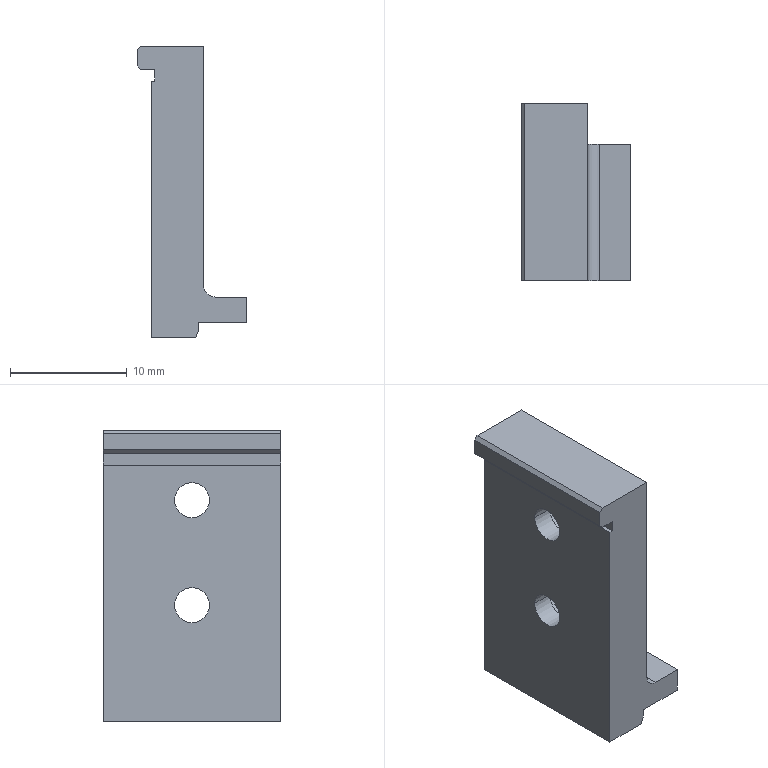Part | NX | 1 solid | 29 faces | box 9.4 x 15.2 x 25 mm | volume 1695 mm3 | plane 20 | cylinder 9 | commonest cylinder face diameters 3 x4 5 x4 2 x1
STEP:
#1=CARTESIAN_POINT('',(-1.77,0.,-1.43));
#2=VERTEX_POINT('',#1);
#3=CARTESIAN_POINT('',(-2.025,0.,-2.13));
#4=VERTEX_POINT('',#3);
#5=CARTESIAN_POINT('',(-1.25,0.,0.));
#6=DIRECTION('',(-0.342,0.,-0.9397));
#7=VECTOR('',#6,1000.);
#8=LINE('',#5,#7);
#9=EDGE_CURVE('',#2,#4,#8,.T.);
#10=ORIENTED_EDGE('',*,*,#9,.T.);
#11=CARTESIAN_POINT('',(-5.85,0.,-2.13));
#12=VERTEX_POINT('',#11);
#13=CARTESIAN_POINT('',(0.,0.,-2.13));
#14=DIRECTION('',(1.,0.,0.));
#15=VECTOR('',#14,1000.);
#16=LINE('',#13,#15);
#17=EDGE_CURVE('',#12,#4,#16,.T.);
#18=ORIENTED_EDGE('',*,*,#17,.F.);
#19=CARTESIAN_POINT('',(-5.85,0.,19.87));
#20=VERTEX_POINT('',#19);
#21=CARTESIAN_POINT('',(-5.85,0.,0.));
#22=DIRECTION('',(0.,0.,1.));
#23=VECTOR('',#22,1000.);
#24=LINE('',#21,#23);
#25=EDGE_CURVE('',#12,#20,#24,.T.);
#26=ORIENTED_EDGE('',*,*,#25,.T.);
#27=CARTESIAN_POINT('',(-5.55,0.,19.87));
#28=VERTEX_POINT('',#27);
#29=CARTESIAN_POINT('',(0.,0.,19.87));
#30=DIRECTION('',(1.,0.,0.));
#31=VECTOR('',#30,1000.);
#32=LINE('',#29,#31);
#33=EDGE_CURVE('',#20,#28,#32,.T.);
#34=ORIENTED_EDGE('',*,*,#33,.T.);
#35=CARTESIAN_POINT('',(-5.55,0.,20.87));
#36=VERTEX_POINT('',#35);
#37=CARTESIAN_POINT('',(-5.55,0.,0.));
#38=DIRECTION('',(0.,0.,1.));
#39=VECTOR('',#38,1000.);
#40=LINE('',#37,#39);
#41=EDGE_CURVE('',#28,#36,#40,.T.);
#42=ORIENTED_EDGE('',*,*,#41,.T.);
#43=CARTESIAN_POINT('',(-6.75,0.,20.87));
#44=VERTEX_POINT('',#43);
#45=CARTESIAN_POINT('',(0.,0.,20.87));
#46=DIRECTION('',(-1.,0.,0.));
#47=VECTOR('',#46,1000.);
#48=LINE('',#45,#47);
#49=EDGE_CURVE('',#36,#44,#48,.T.);
#50=ORIENTED_EDGE('',*,*,#49,.T.);
#51=CARTESIAN_POINT('',(-7.05,0.,21.17));
#52=VERTEX_POINT('',#51);
#53=CARTESIAN_POINT('',(14.12,0.,0.));
#54=DIRECTION('',(0.7071,0.,-0.7071));
#55=VECTOR('',#54,1000.);
#56=LINE('',#53,#55);
#57=EDGE_CURVE('',#52,#44,#56,.T.);
#58=ORIENTED_EDGE('',*,*,#57,.F.);
#59=CARTESIAN_POINT('',(-7.05,0.,22.57));
#60=VERTEX_POINT('',#59);
#61=CARTESIAN_POINT('',(-7.05,0.,0.));
#62=DIRECTION('',(0.,0.,1.));
#63=VECTOR('',#62,1000.);
#64=LINE('',#61,#63);
#65=EDGE_CURVE('',#52,#60,#64,.T.);
#66=ORIENTED_EDGE('',*,*,#65,.T.);
#67=CARTESIAN_POINT('',(-6.75,0.,22.87));
#68=VERTEX_POINT('',#67);
#69=CARTESIAN_POINT('',(-29.62,0.,0.));
#70=DIRECTION('',(0.7071,0.,0.7071));
#71=VECTOR('',#70,1000.);
#72=LINE('',#69,#71);
#73=EDGE_CURVE('',#60,#68,#72,.T.);
#74=ORIENTED_EDGE('',*,*,#73,.T.);
#75=CARTESIAN_POINT('',(-1.35,0.,22.87));
#76=VERTEX_POINT('',#75);
#77=CARTESIAN_POINT('',(0.,0.,22.87));
#78=DIRECTION('',(1.,0.,0.));
#79=VECTOR('',#78,1000.);
#80=LINE('',#77,#79);
#81=EDGE_CURVE('',#68,#76,#80,.T.);
#82=ORIENTED_EDGE('',*,*,#81,.T.);
#83=CARTESIAN_POINT('',(-1.35,0.,-0.78));
#84=VERTEX_POINT('',#83);
#85=CARTESIAN_POINT('',(-1.35,0.,0.));
#86=DIRECTION('',(0.,0.,-1.));
#87=VECTOR('',#86,1000.);
#88=LINE('',#85,#87);
#89=EDGE_CURVE('',#76,#84,#88,.T.);
#90=ORIENTED_EDGE('',*,*,#89,.T.);
#91=CARTESIAN_POINT('',(-1.77,0.,-0.78));
#92=VERTEX_POINT('',#91);
#93=CARTESIAN_POINT('',(0.,0.,-0.78));
#94=DIRECTION('',(1.,0.,0.));
#95=VECTOR('',#94,1000.);
#96=LINE('',#93,#95);
#97=EDGE_CURVE('',#92,#84,#96,.T.);
#98=ORIENTED_EDGE('',*,*,#97,.F.);
#99=CARTESIAN_POINT('',(-1.77,0.,0.));
#100=DIRECTION('',(0.,0.,1.));
#101=VECTOR('',#100,1000.);
#102=LINE('',#99,#101);
#103=EDGE_CURVE('',#2,#92,#102,.T.);
#104=ORIENTED_EDGE('',*,*,#103,.F.);
#105=EDGE_LOOP('',(#10,#18,#26,#34,#42,#50,#58,#66,#74,#82,#90,#98,#104));
#106=FACE_BOUND('',#105,.T.);
#107=CARTESIAN_POINT('',(0.,0.,0.));
#108=DIRECTION('',(0.,-1.,0.));
#109=DIRECTION('',(0.,0.,-1.));
#110=AXIS2_PLACEMENT_3D('',#107,#108,#109);
#111=PLANE('',#110);
#112=ADVANCED_FACE('',(#106),#111,.F.);
#113=CARTESIAN_POINT('',(-1.77,-15.2,-1.43));
#114=VERTEX_POINT('',#113);
#115=CARTESIAN_POINT('',(-1.77,0.,-1.43));
#116=DIRECTION('',(0.,-1.,0.));
#117=VECTOR('',#116,1000.);
#118=LINE('',#115,#117);
#119=EDGE_CURVE('',#2,#114,#118,.T.);
#120=ORIENTED_EDGE('',*,*,#119,.F.);
#121=ORIENTED_EDGE('',*,*,#103,.T.);
#122=CARTESIAN_POINT('',(-1.77,-15.2,-0.78));
#123=VERTEX_POINT('',#122);
#124=CARTESIAN_POINT('',(-1.77,0.,-0.78));
#125=DIRECTION('',(0.,1.,0.));
#126=VECTOR('',#125,1000.);
#127=LINE('',#124,#126);
#128=EDGE_CURVE('',#123,#92,#127,.T.);
#129=ORIENTED_EDGE('',*,*,#128,.F.);
#130=CARTESIAN_POINT('',(-1.77,-15.2,0.));
#131=DIRECTION('',(0.,0.,1.));
#132=VECTOR('',#131,1000.);
#133=LINE('',#130,#132);
#134=EDGE_CURVE('',#114,#123,#133,.T.);
#135=ORIENTED_EDGE('',*,*,#134,.F.);
#136=EDGE_LOOP('',(#120,#121,#129,#135));
#137=FACE_BOUND('',#136,.T.);
#138=CARTESIAN_POINT('',(-1.77,0.,-0.93));
#139=DIRECTION('',(1.,0.,0.));
#140=DIRECTION('',(0.,1.,0.));
#141=AXIS2_PLACEMENT_3D('',#138,#139,#140);
#142=PLANE('',#141);
#143=ADVANCED_FACE('',(#137),#142,.T.);
#144=CARTESIAN_POINT('',(-0.35,-15.2,1.37));
#145=VERTEX_POINT('',#144);
#146=CARTESIAN_POINT('',(2.35,-15.2,1.37));
#147=VERTEX_POINT('',#146);
#148=CARTESIAN_POINT('',(0.,-15.2,1.37));
#149=DIRECTION('',(1.,0.,0.));
#150=VECTOR('',#149,1000.);
#151=LINE('',#148,#150);
#152=EDGE_CURVE('',#145,#147,#151,.T.);
#153=ORIENTED_EDGE('',*,*,#152,.F.);
#154=CARTESIAN_POINT('',(-1.35,-15.2,2.37));
#155=VERTEX_POINT('',#154);
#156=CARTESIAN_POINT('',(-0.35,-15.2,2.37));
#157=DIRECTION('',(0.,1.,0.));
#158=DIRECTION('',(-1.,0.,0.));
#159=AXIS2_PLACEMENT_3D('',#156,#157,#158);
#160=CIRCLE('',#159,1.);
#161=EDGE_CURVE('',#145,#155,#160,.T.);
#162=ORIENTED_EDGE('',*,*,#161,.T.);
#163=CARTESIAN_POINT('',(-1.35,-15.2,22.87));
#164=VERTEX_POINT('',#163);
#165=CARTESIAN_POINT('',(-1.35,-15.2,0.));
#166=DIRECTION('',(0.,0.,-1.));
#167=VECTOR('',#166,1000.);
#168=LINE('',#165,#167);
#169=EDGE_CURVE('',#164,#155,#168,.T.);
#170=ORIENTED_EDGE('',*,*,#169,.F.);
#171=CARTESIAN_POINT('',(-6.75,-15.2,22.87));
#172=VERTEX_POINT('',#171);
#173=CARTESIAN_POINT('',(0.,-15.2,22.87));
#174=DIRECTION('',(-1.,0.,0.));
#175=VECTOR('',#174,1000.);
#176=LINE('',#173,#175);
#177=EDGE_CURVE('',#164,#172,#176,.T.);
#178=ORIENTED_EDGE('',*,*,#177,.T.);
#179=CARTESIAN_POINT('',(-7.05,-15.2,22.57));
#180=VERTEX_POINT('',#179);
#181=CARTESIAN_POINT('',(-29.62,-15.2,0.));
#182=DIRECTION('',(-0.7071,0.,-0.7071));
#183=VECTOR('',#182,1000.);
#184=LINE('',#181,#183);
#185=EDGE_CURVE('',#172,#180,#184,.T.);
#186=ORIENTED_EDGE('',*,*,#185,.T.);
#187=CARTESIAN_POINT('',(-7.05,-15.2,21.17));
#188=VERTEX_POINT('',#187);
#189=CARTESIAN_POINT('',(-7.05,-15.2,0.));
#190=DIRECTION('',(0.,0.,-1.));
#191=VECTOR('',#190,1000.);
#192=LINE('',#189,#191);
#193=EDGE_CURVE('',#180,#188,#192,.T.);
#194=ORIENTED_EDGE('',*,*,#193,.T.);
#195=CARTESIAN_POINT('',(-6.75,-15.2,20.87));
#196=VERTEX_POINT('',#195);
#197=CARTESIAN_POINT('',(14.12,-15.2,0.));
#198=DIRECTION('',(-0.7071,0.,0.7071));
#199=VECTOR('',#198,1000.);
#200=LINE('',#197,#199);
#201=EDGE_CURVE('',#196,#188,#200,.T.);
#202=ORIENTED_EDGE('',*,*,#201,.F.);
#203=CARTESIAN_POINT('',(-5.55,-15.2,20.87));
#204=VERTEX_POINT('',#203);
#205=CARTESIAN_POINT('',(0.,-15.2,20.87));
#206=DIRECTION('',(1.,0.,0.));
#207=VECTOR('',#206,1000.);
#208=LINE('',#205,#207);
#209=EDGE_CURVE('',#196,#204,#208,.T.);
#210=ORIENTED_EDGE('',*,*,#209,.T.);
#211=CARTESIAN_POINT('',(-5.55,-15.2,19.87));
#212=VERTEX_POINT('',#211);
#213=CARTESIAN_POINT('',(-5.55,-15.2,0.));
#214=DIRECTION('',(0.,0.,-1.));
#215=VECTOR('',#214,1000.);
#216=LINE('',#213,#215);
#217=EDGE_CURVE('',#204,#212,#216,.T.);
#218=ORIENTED_EDGE('',*,*,#217,.T.);
#219=CARTESIAN_POINT('',(-5.85,-15.2,19.87));
#220=VERTEX_POINT('',#219);
#221=CARTESIAN_POINT('',(0.,-15.2,19.87));
#222=DIRECTION('',(-1.,0.,0.));
#223=VECTOR('',#222,1000.);
#224=LINE('',#221,#223);
#225=EDGE_CURVE('',#212,#220,#224,.T.);
#226=ORIENTED_EDGE('',*,*,#225,.T.);
#227=CARTESIAN_POINT('',(-5.85,-15.2,-2.13));
#228=VERTEX_POINT('',#227);
#229=CARTESIAN_POINT('',(-5.85,-15.2,0.));
#230=DIRECTION('',(0.,0.,-1.));
#231=VECTOR('',#230,1000.);
#232=LINE('',#229,#231);
#233=EDGE_CURVE('',#220,#228,#232,.T.);
#234=ORIENTED_EDGE('',*,*,#233,.T.);
#235=CARTESIAN_POINT('',(-2.025,-15.2,-2.13));
#236=VERTEX_POINT('',#235);
#237=CARTESIAN_POINT('',(0.,-15.2,-2.13));
#238=DIRECTION('',(-1.,0.,0.));
#239=VECTOR('',#238,1000.);
#240=LINE('',#237,#239);
#241=EDGE_CURVE('',#236,#228,#240,.T.);
#242=ORIENTED_EDGE('',*,*,#241,.F.);
#243=CARTESIAN_POINT('',(-1.25,-15.2,0.));
#244=DIRECTION('',(0.342,0.,0.9397));
#245=VECTOR('',#244,1000.);
#246=LINE('',#243,#245);
#247=EDGE_CURVE('',#236,#114,#246,.T.);
#248=ORIENTED_EDGE('',*,*,#247,.T.);
#249=ORIENTED_EDGE('',*,*,#134,.T.);
#250=CARTESIAN_POINT('',(2.35,-15.2,-0.78));
#251=VERTEX_POINT('',#250);
#252=CARTESIAN_POINT('',(0.,-15.2,-0.78));
#253=DIRECTION('',(-1.,0.,0.));
#254=VECTOR('',#253,1000.);
#255=LINE('',#252,#254);
#256=EDGE_CURVE('',#251,#123,#255,.T.);
#257=ORIENTED_EDGE('',*,*,#256,.F.);
#258=CARTESIAN_POINT('',(2.35,-15.2,0.));
#259=DIRECTION('',(0.,0.,1.));
#260=VECTOR('',#259,1000.);
#261=LINE('',#258,#260);
#262=EDGE_CURVE('',#251,#147,#261,.T.);
#263=ORIENTED_EDGE('',*,*,#262,.T.);
#264=EDGE_LOOP('',(#153,#162,#170,#178,#186,#194,#202,#210,#218,#226,#234,#242,#248,#249,#257,#263));
#265=FACE_BOUND('',#264,.T.);
#266=CARTESIAN_POINT('',(-1.35,-15.2,0.));
#267=DIRECTION('',(0.,1.,0.));
#268=DIRECTION('',(1.,0.,0.));
#269=AXIS2_PLACEMENT_3D('',#266,#267,#268);
#270=PLANE('',#269);
#271=ADVANCED_FACE('',(#265),#270,.F.);
#272=CARTESIAN_POINT('',(-4.05,-5.1,7.87));
#273=VERTEX_POINT('',#272);
#274=CARTESIAN_POINT('',(-4.05,-10.1,7.87));
#275=VERTEX_POINT('',#274);
#276=CARTESIAN_POINT('',(-4.05,-7.6,7.87));
#277=DIRECTION('',(1.,0.,0.));
#278=DIRECTION('',(0.,-1.,0.));
#279=AXIS2_PLACEMENT_3D('',#276,#277,#278);
#280=CIRCLE('',#279,2.5);
#281=EDGE_CURVE('',#273,#275,#280,.T.);
#282=ORIENTED_EDGE('',*,*,#281,.T.);
#283=CARTESIAN_POINT('',(-4.05,-7.6,7.87));
#284=DIRECTION('',(1.,0.,0.));
#285=DIRECTION('',(0.,-1.,0.));
#286=AXIS2_PLACEMENT_3D('',#283,#284,#285);
#287=CIRCLE('',#286,2.5);
#288=EDGE_CURVE('',#275,#273,#287,.T.);
#289=ORIENTED_EDGE('',*,*,#288,.T.);
#290=EDGE_LOOP('',(#282,#289));
#291=FACE_BOUND('',#290,.T.);
#292=CARTESIAN_POINT('',(-4.05,-6.1,7.87));
#293=VERTEX_POINT('',#292);
#294=CARTESIAN_POINT('',(-4.05,-9.1,7.87));
#295=VERTEX_POINT('',#294);
#296=CARTESIAN_POINT('',(-4.05,-7.6,7.87));
#297=DIRECTION('',(1.,0.,0.));
#298=DIRECTION('',(0.,-1.,0.));
#299=AXIS2_PLACEMENT_3D('',#296,#297,#298);
#300=CIRCLE('',#299,1.5);
#301=EDGE_CURVE('',#293,#295,#300,.T.);
#302=ORIENTED_EDGE('',*,*,#301,.F.);
#303=CARTESIAN_POINT('',(-4.05,-7.6,7.87));
#304=DIRECTION('',(1.,0.,0.));
#305=DIRECTION('',(0.,-1.,0.));
#306=AXIS2_PLACEMENT_3D('',#303,#304,#305);
#307=CIRCLE('',#306,1.5);
#308=EDGE_CURVE('',#295,#293,#307,.T.);
#309=ORIENTED_EDGE('',*,*,#308,.F.);
#310=EDGE_LOOP('',(#302,#309));
#311=FACE_BOUND('',#310,.T.);
#312=CARTESIAN_POINT('',(-4.05,-7.6,7.87));
#313=DIRECTION('',(-1.,0.,0.));
#314=DIRECTION('',(0.,0.,1.));
#315=AXIS2_PLACEMENT_3D('',#312,#313,#314);
#316=PLANE('',#315);
#317=ADVANCED_FACE('',(#291,#311),#316,.F.);
#318=ORIENTED_EDGE('',*,*,#241,.T.);
#319=CARTESIAN_POINT('',(-5.85,0.,-2.13));
#320=DIRECTION('',(0.,1.,0.));
#321=VECTOR('',#320,1000.);
#322=LINE('',#319,#321);
#323=EDGE_CURVE('',#228,#12,#322,.T.);
#324=ORIENTED_EDGE('',*,*,#323,.T.);
#325=ORIENTED_EDGE('',*,*,#17,.T.);
#326=CARTESIAN_POINT('',(-2.025,0.,-2.13));
#327=DIRECTION('',(0.,-1.,0.));
#328=VECTOR('',#327,1000.);
#329=LINE('',#326,#328);
#330=EDGE_CURVE('',#4,#236,#329,.T.);
#331=ORIENTED_EDGE('',*,*,#330,.T.);
#332=EDGE_LOOP('',(#318,#324,#325,#331));
#333=FACE_BOUND('',#332,.T.);
#334=CARTESIAN_POINT('',(0.,0.,-2.13));
#335=DIRECTION('',(0.,0.,1.));
#336=DIRECTION('',(1.,0.,0.));
#337=AXIS2_PLACEMENT_3D('',#334,#335,#336);
#338=PLANE('',#337);
#339=ADVANCED_FACE('',(#333),#338,.F.);
#340=ORIENTED_EDGE('',*,*,#9,.F.);
#341=ORIENTED_EDGE('',*,*,#119,.T.);
#342=ORIENTED_EDGE('',*,*,#247,.F.);
#343=ORIENTED_EDGE('',*,*,#330,.F.);
#344=EDGE_LOOP('',(#340,#341,#342,#343));
#345=FACE_BOUND('',#344,.T.);
#346=CARTESIAN_POINT('',(-2.025,-15.2,-2.13));
#347=DIRECTION('',(0.9397,0.,-0.342));
#348=DIRECTION('',(0.,-1.,0.));
#349=AXIS2_PLACEMENT_3D('',#346,#347,#348);
#350=PLANE('',#349);
#351=ADVANCED_FACE('',(#345),#350,.T.);
#352=CARTESIAN_POINT('',(-5.85,0.,19.87));
#353=DIRECTION('',(0.,-1.,0.));
#354=VECTOR('',#353,1000.);
#355=LINE('',#352,#354);
#356=EDGE_CURVE('',#20,#220,#355,.T.);
#357=ORIENTED_EDGE('',*,*,#356,.T.);
#358=ORIENTED_EDGE('',*,*,#225,.F.);
#359=CARTESIAN_POINT('',(-5.55,0.,19.87));
#360=DIRECTION('',(0.,-1.,0.));
#361=VECTOR('',#360,1000.);
#362=LINE('',#359,#361);
#363=EDGE_CURVE('',#28,#212,#362,.T.);
#364=ORIENTED_EDGE('',*,*,#363,.F.);
#365=ORIENTED_EDGE('',*,*,#33,.F.);
#366=EDGE_LOOP('',(#357,#358,#364,#365));
#367=FACE_BOUND('',#366,.T.);
#368=CARTESIAN_POINT('',(-4.85,0.,19.87));
#369=DIRECTION('',(0.,0.,1.));
#370=DIRECTION('',(1.,0.,0.));
#371=AXIS2_PLACEMENT_3D('',#368,#369,#370);
#372=PLANE('',#371);
#373=ADVANCED_FACE('',(#367),#372,.T.);
#374=ORIENTED_EDGE('',*,*,#363,.T.);
#375=ORIENTED_EDGE('',*,*,#217,.F.);
#376=CARTESIAN_POINT('',(-5.55,0.,20.87));
#377=DIRECTION('',(0.,-1.,0.));
#378=VECTOR('',#377,1000.);
#379=LINE('',#376,#378);
#380=EDGE_CURVE('',#36,#204,#379,.T.);
#381=ORIENTED_EDGE('',*,*,#380,.F.);
#382=ORIENTED_EDGE('',*,*,#41,.F.);
#383=EDGE_LOOP('',(#374,#375,#381,#382));
#384=FACE_BOUND('',#383,.T.);
#385=CARTESIAN_POINT('',(-5.55,0.,19.87));
#386=DIRECTION('',(-1.,0.,0.));
#387=DIRECTION('',(0.,0.,1.));
#388=AXIS2_PLACEMENT_3D('',#385,#386,#387);
#389=PLANE('',#388);
#390=ADVANCED_FACE('',(#384),#389,.T.);
#391=CARTESIAN_POINT('',(-6.75,0.,20.87));
#392=DIRECTION('',(0.,1.,0.));
#393=VECTOR('',#392,1000.);
#394=LINE('',#391,#393);
#395=EDGE_CURVE('',#196,#44,#394,.T.);
#396=ORIENTED_EDGE('',*,*,#395,.T.);
#397=ORIENTED_EDGE('',*,*,#49,.F.);
#398=ORIENTED_EDGE('',*,*,#380,.T.);
#399=ORIENTED_EDGE('',*,*,#209,.F.);
#400=EDGE_LOOP('',(#396,#397,#398,#399));
#401=FACE_BOUND('',#400,.T.);
#402=CARTESIAN_POINT('',(-4.85,0.,20.87));
#403=DIRECTION('',(0.,0.,-1.));
#404=DIRECTION('',(0.,-1.,0.));
#405=AXIS2_PLACEMENT_3D('',#402,#403,#404);
#406=PLANE('',#405);
#407=ADVANCED_FACE('',(#401),#406,.T.);
#408=CARTESIAN_POINT('',(-7.05,0.,22.57));
#409=DIRECTION('',(0.,-1.,0.));
#410=VECTOR('',#409,1000.);
#411=LINE('',#408,#410);
#412=EDGE_CURVE('',#60,#180,#411,.T.);
#413=ORIENTED_EDGE('',*,*,#412,.F.);
#414=ORIENTED_EDGE('',*,*,#65,.F.);
#415=CARTESIAN_POINT('',(-7.05,0.,21.17));
#416=DIRECTION('',(0.,-1.,0.));
#417=VECTOR('',#416,1000.);
#418=LINE('',#415,#417);
#419=EDGE_CURVE('',#52,#188,#418,.T.);
#420=ORIENTED_EDGE('',*,*,#419,.T.);
#421=ORIENTED_EDGE('',*,*,#193,.F.);
#422=EDGE_LOOP('',(#413,#414,#420,#421));
#423=FACE_BOUND('',#422,.T.);
#424=CARTESIAN_POINT('',(-7.05,0.,20.87));
#425=DIRECTION('',(-1.,0.,0.));
#426=DIRECTION('',(0.,0.,1.));
#427=AXIS2_PLACEMENT_3D('',#424,#425,#426);
#428=PLANE('',#427);
#429=ADVANCED_FACE('',(#423),#428,.T.);
#430=CARTESIAN_POINT('',(-6.75,0.,22.87));
#431=DIRECTION('',(0.,1.,0.));
#432=VECTOR('',#431,1000.);
#433=LINE('',#430,#432);
#434=EDGE_CURVE('',#172,#68,#433,.T.);
#435=ORIENTED_EDGE('',*,*,#434,.F.);
#436=ORIENTED_EDGE('',*,*,#177,.F.);
#437=CARTESIAN_POINT('',(-1.35,0.,22.87));
#438=DIRECTION('',(0.,-1.,0.));
#439=VECTOR('',#438,1000.);
#440=LINE('',#437,#439);
#441=EDGE_CURVE('',#76,#164,#440,.T.);
#442=ORIENTED_EDGE('',*,*,#441,.F.);
#443=ORIENTED_EDGE('',*,*,#81,.F.);
#444=EDGE_LOOP('',(#435,#436,#442,#443));
#445=FACE_BOUND('',#444,.T.);
#446=CARTESIAN_POINT('',(-6.05,0.,22.87));
#447=DIRECTION('',(0.,0.,1.));
#448=DIRECTION('',(1.,0.,0.));
#449=AXIS2_PLACEMENT_3D('',#446,#447,#448);
#450=PLANE('',#449);
#451=ADVANCED_FACE('',(#445),#450,.T.);
#452=ORIENTED_EDGE('',*,*,#169,.T.);
#453=CARTESIAN_POINT('',(-1.35,-3.5,2.37));
#454=VERTEX_POINT('',#453);
#455=CARTESIAN_POINT('',(-1.35,-15.285,2.37));
#456=DIRECTION('',(0.,1.,0.));
#457=VECTOR('',#456,1000.);
#458=LINE('',#455,#457);
#459=EDGE_CURVE('',#155,#454,#458,.T.);
#460=ORIENTED_EDGE('',*,*,#459,.T.);
#461=CARTESIAN_POINT('',(-1.35,-3.5,-0.78));
#462=VERTEX_POINT('',#461);
#463=CARTESIAN_POINT('',(-1.35,-3.5,0.));
#464=DIRECTION('',(0.,0.,-1.));
#465=VECTOR('',#464,1000.);
#466=LINE('',#463,#465);
#467=EDGE_CURVE('',#454,#462,#466,.T.);
#468=ORIENTED_EDGE('',*,*,#467,.T.);
#469=CARTESIAN_POINT('',(-1.35,0.,-0.78));
#470=DIRECTION('',(0.,-1.,0.));
#471=VECTOR('',#470,1000.);
#472=LINE('',#469,#471);
#473=EDGE_CURVE('',#84,#462,#472,.T.);
#474=ORIENTED_EDGE('',*,*,#473,.F.);
#475=ORIENTED_EDGE('',*,*,#89,.F.);
#476=ORIENTED_EDGE('',*,*,#441,.T.);
#477=EDGE_LOOP('',(#452,#460,#468,#474,#475,#476));
#478=FACE_BOUND('',#477,.T.);
#479=CARTESIAN_POINT('',(-1.35,-10.1,16.87));
#480=VERTEX_POINT('',#479);
#481=CARTESIAN_POINT('',(-1.35,-5.1,16.87));
#482=VERTEX_POINT('',#481);
#483=CARTESIAN_POINT('',(-1.35,-7.6,16.87));
#484=DIRECTION('',(1.,0.,0.));
#485=DIRECTION('',(0.,-1.,0.));
#486=AXIS2_PLACEMENT_3D('',#483,#484,#485);
#487=CIRCLE('',#486,2.5);
#488=EDGE_CURVE('',#480,#482,#487,.T.);
#489=ORIENTED_EDGE('',*,*,#488,.F.);
#490=CARTESIAN_POINT('',(-1.35,-7.6,16.87));
#491=DIRECTION('',(1.,0.,0.));
#492=DIRECTION('',(0.,-1.,0.));
#493=AXIS2_PLACEMENT_3D('',#490,#491,#492);
#494=CIRCLE('',#493,2.5);
#495=EDGE_CURVE('',#482,#480,#494,.T.);
#496=ORIENTED_EDGE('',*,*,#495,.F.);
#497=EDGE_LOOP('',(#489,#496));
#498=FACE_BOUND('',#497,.T.);
#499=CARTESIAN_POINT('',(-1.35,-5.1,7.87));
#500=VERTEX_POINT('',#499);
#501=CARTESIAN_POINT('',(-1.35,-10.1,7.87));
#502=VERTEX_POINT('',#501);
#503=CARTESIAN_POINT('',(-1.35,-7.6,7.87));
#504=DIRECTION('',(1.,0.,0.));
#505=DIRECTION('',(0.,-1.,0.));
#506=AXIS2_PLACEMENT_3D('',#503,#504,#505);
#507=CIRCLE('',#506,2.5);
#508=EDGE_CURVE('',#500,#502,#507,.T.);
#509=ORIENTED_EDGE('',*,*,#508,.F.);
#510=CARTESIAN_POINT('',(-1.35,-7.6,7.87));
#511=DIRECTION('',(1.,0.,0.));
#512=DIRECTION('',(0.,-1.,0.));
#513=AXIS2_PLACEMENT_3D('',#510,#511,#512);
#514=CIRCLE('',#513,2.5);
#515=EDGE_CURVE('',#502,#500,#514,.T.);
#516=ORIENTED_EDGE('',*,*,#515,.F.);
#517=EDGE_LOOP('',(#509,#516));
#518=FACE_BOUND('',#517,.T.);
#519=CARTESIAN_POINT('',(-1.35,0.,-1.13));
#520=DIRECTION('',(-1.,0.,0.));
#521=DIRECTION('',(0.,0.,1.));
#522=AXIS2_PLACEMENT_3D('',#519,#520,#521);
#523=PLANE('',#522);
#524=ADVANCED_FACE('',(#478,#498,#518),#523,.F.);
#525=ORIENTED_EDGE('',*,*,#459,.F.);
#526=ORIENTED_EDGE('',*,*,#161,.F.);
#527=CARTESIAN_POINT('',(-0.35,-3.5,1.37));
#528=VERTEX_POINT('',#527);
#529=CARTESIAN_POINT('',(-0.35,-15.2,1.37));
#530=DIRECTION('',(0.,1.,0.));
#531=VECTOR('',#530,1000.);
#532=LINE('',#529,#531);
#533=EDGE_CURVE('',#145,#528,#532,.T.);
#534=ORIENTED_EDGE('',*,*,#533,.T.);
#535=CARTESIAN_POINT('',(-0.35,-3.5,2.37));
#536=DIRECTION('',(0.,1.,0.));
#537=DIRECTION('',(-1.,0.,0.));
#538=AXIS2_PLACEMENT_3D('',#535,#536,#537);
#539=CIRCLE('',#538,1.);
#540=EDGE_CURVE('',#528,#454,#539,.T.);
#541=ORIENTED_EDGE('',*,*,#540,.T.);
#542=EDGE_LOOP('',(#525,#526,#534,#541));
#543=FACE_BOUND('',#542,.T.);
#544=CARTESIAN_POINT('',(-0.35,-15.285,2.37));
#545=DIRECTION('',(0.,1.,0.));
#546=DIRECTION('',(-1.,0.,0.));
#547=AXIS2_PLACEMENT_3D('',#544,#545,#546);
#548=CYLINDRICAL_SURFACE('',#547,1.);
#549=ADVANCED_FACE('',(#543),#548,.F.);
#550=CARTESIAN_POINT('',(2.35,-3.5,1.37));
#551=VERTEX_POINT('',#550);
#552=CARTESIAN_POINT('',(2.35,-3.5,-0.78));
#553=VERTEX_POINT('',#552);
#554=CARTESIAN_POINT('',(2.35,-3.5,0.));
#555=DIRECTION('',(0.,0.,-1.));
#556=VECTOR('',#555,1000.);
#557=LINE('',#554,#556);
#558=EDGE_CURVE('',#551,#553,#557,.T.);
#559=ORIENTED_EDGE('',*,*,#558,.T.);
#560=CARTESIAN_POINT('',(0.,-3.5,-0.78));
#561=DIRECTION('',(1.,0.,0.));
#562=VECTOR('',#561,1000.);
#563=LINE('',#560,#562);
#564=EDGE_CURVE('',#462,#553,#563,.T.);
#565=ORIENTED_EDGE('',*,*,#564,.F.);
#566=ORIENTED_EDGE('',*,*,#467,.F.);
#567=ORIENTED_EDGE('',*,*,#540,.F.);
#568=CARTESIAN_POINT('',(0.,-3.5,1.37));
#569=DIRECTION('',(-1.,0.,0.));
#570=VECTOR('',#569,1000.);
#571=LINE('',#568,#570);
#572=EDGE_CURVE('',#551,#528,#571,.T.);
#573=ORIENTED_EDGE('',*,*,#572,.F.);
#574=EDGE_LOOP('',(#559,#565,#566,#567,#573));
#575=FACE_BOUND('',#574,.T.);
#576=CARTESIAN_POINT('',(-1.77,-3.5,-0.83));
#577=DIRECTION('',(0.,-1.,0.));
#578=DIRECTION('',(0.,0.,-1.));
#579=AXIS2_PLACEMENT_3D('',#576,#577,#578);
#580=PLANE('',#579);
#581=ADVANCED_FACE('',(#575),#580,.F.);
#582=ORIENTED_EDGE('',*,*,#262,.F.);
#583=CARTESIAN_POINT('',(2.35,0.,-0.78));
#584=DIRECTION('',(0.,1.,0.));
#585=VECTOR('',#584,1000.);
#586=LINE('',#583,#585);
#587=EDGE_CURVE('',#251,#553,#586,.T.);
#588=ORIENTED_EDGE('',*,*,#587,.T.);
#589=ORIENTED_EDGE('',*,*,#558,.F.);
#590=CARTESIAN_POINT('',(2.35,0.,1.37));
#591=DIRECTION('',(0.,1.,0.));
#592=VECTOR('',#591,1000.);
#593=LINE('',#590,#592);
#594=EDGE_CURVE('',#147,#551,#593,.T.);
#595=ORIENTED_EDGE('',*,*,#594,.F.);
#596=EDGE_LOOP('',(#582,#588,#589,#595));
#597=FACE_BOUND('',#596,.T.);
#598=CARTESIAN_POINT('',(2.35,0.,52.77));
#599=DIRECTION('',(-1.,0.,0.));
#600=DIRECTION('',(0.,0.,1.));
#601=AXIS2_PLACEMENT_3D('',#598,#599,#600);
#602=PLANE('',#601);
#603=ADVANCED_FACE('',(#597),#602,.F.);
#604=ORIENTED_EDGE('',*,*,#508,.T.);
#605=CARTESIAN_POINT('',(-7.072,-10.1,7.87));
#606=DIRECTION('',(1.,0.,0.));
#607=VECTOR('',#606,1000.);
#608=LINE('',#605,#607);
#609=EDGE_CURVE('',#502,#275,#608,.F.);
#610=ORIENTED_EDGE('',*,*,#609,.T.);
#611=ORIENTED_EDGE('',*,*,#281,.F.);
#612=CARTESIAN_POINT('',(-7.072,-5.1,7.87));
#613=DIRECTION('',(1.,0.,0.));
#614=VECTOR('',#613,1000.);
#615=LINE('',#612,#614);
#616=EDGE_CURVE('',#500,#273,#615,.F.);
#617=ORIENTED_EDGE('',*,*,#616,.F.);
#618=EDGE_LOOP('',(#604,#610,#611,#617));
#619=FACE_BOUND('',#618,.T.);
#620=CARTESIAN_POINT('',(-7.072,-7.6,7.87));
#621=DIRECTION('',(1.,0.,0.));
#622=DIRECTION('',(0.,-1.,0.));
#623=AXIS2_PLACEMENT_3D('',#620,#621,#622);
#624=CYLINDRICAL_SURFACE('',#623,2.5);
#625=ADVANCED_FACE('',(#619),#624,.F.);
#626=ORIENTED_EDGE('',*,*,#572,.T.);
#627=ORIENTED_EDGE('',*,*,#533,.F.);
#628=ORIENTED_EDGE('',*,*,#152,.T.);
#629=ORIENTED_EDGE('',*,*,#594,.T.);
#630=EDGE_LOOP('',(#626,#627,#628,#629));
#631=FACE_BOUND('',#630,.T.);
#632=CARTESIAN_POINT('',(-1.35,-15.2,1.37));
#633=DIRECTION('',(0.,0.,-1.));
#634=DIRECTION('',(0.,-1.,0.));
#635=AXIS2_PLACEMENT_3D('',#632,#633,#634);
#636=PLANE('',#635);
#637=ADVANCED_FACE('',(#631),#636,.F.);
#638=ORIENTED_EDGE('',*,*,#97,.T.);
#639=ORIENTED_EDGE('',*,*,#473,.T.);
#640=ORIENTED_EDGE('',*,*,#564,.T.);
#641=ORIENTED_EDGE('',*,*,#587,.F.);
#642=ORIENTED_EDGE('',*,*,#256,.T.);
#643=ORIENTED_EDGE('',*,*,#128,.T.);
#644=EDGE_LOOP('',(#638,#639,#640,#641,#642,#643));
#645=FACE_BOUND('',#644,.T.);
#646=CARTESIAN_POINT('',(1.45,0.,-0.78));
#647=DIRECTION('',(0.,0.,-1.));
#648=DIRECTION('',(0.,-1.,0.));
#649=AXIS2_PLACEMENT_3D('',#646,#647,#648);
#650=PLANE('',#649);
#651=ADVANCED_FACE('',(#645),#650,.T.);
#652=ORIENTED_EDGE('',*,*,#395,.F.);
#653=ORIENTED_EDGE('',*,*,#201,.T.);
#654=ORIENTED_EDGE('',*,*,#419,.F.);
#655=ORIENTED_EDGE('',*,*,#57,.T.);
#656=EDGE_LOOP('',(#652,#653,#654,#655));
#657=FACE_BOUND('',#656,.T.);
#658=CARTESIAN_POINT('',(-6.9,-7.6,21.02));
#659=DIRECTION('',(0.7071,0.,0.7071));
#660=DIRECTION('',(0.,-1.,0.));
#661=AXIS2_PLACEMENT_3D('',#658,#659,#660);
#662=PLANE('',#661);
#663=ADVANCED_FACE('',(#657),#662,.F.);
#664=ORIENTED_EDGE('',*,*,#412,.T.);
#665=ORIENTED_EDGE('',*,*,#185,.F.);
#666=ORIENTED_EDGE('',*,*,#434,.T.);
#667=ORIENTED_EDGE('',*,*,#73,.F.);
#668=EDGE_LOOP('',(#664,#665,#666,#667));
#669=FACE_BOUND('',#668,.T.);
#670=CARTESIAN_POINT('',(-6.9,-7.6,22.72));
#671=DIRECTION('',(-0.7071,0.,0.7071));
#672=DIRECTION('',(0.,1.,0.));
#673=AXIS2_PLACEMENT_3D('',#670,#671,#672);
#674=PLANE('',#673);
#675=ADVANCED_FACE('',(#669),#674,.T.);
#676=ORIENTED_EDGE('',*,*,#488,.T.);
#677=CARTESIAN_POINT('',(-4.05,-5.1,16.87));
#678=VERTEX_POINT('',#677);
#679=CARTESIAN_POINT('',(-7.072,-5.1,16.87));
#680=DIRECTION('',(1.,0.,0.));
#681=VECTOR('',#680,1000.);
#682=LINE('',#679,#681);
#683=EDGE_CURVE('',#678,#482,#682,.T.);
#684=ORIENTED_EDGE('',*,*,#683,.F.);
#685=CARTESIAN_POINT('',(-4.05,-10.1,16.87));
#686=VERTEX_POINT('',#685);
#687=CARTESIAN_POINT('',(-4.05,-7.6,16.87));
#688=DIRECTION('',(1.,0.,0.));
#689=DIRECTION('',(0.,-1.,0.));
#690=AXIS2_PLACEMENT_3D('',#687,#688,#689);
#691=CIRCLE('',#690,2.5);
#692=EDGE_CURVE('',#686,#678,#691,.T.);
#693=ORIENTED_EDGE('',*,*,#692,.F.);
#694=CARTESIAN_POINT('',(-7.072,-10.1,16.87));
#695=DIRECTION('',(1.,0.,0.));
#696=VECTOR('',#695,1000.);
#697=LINE('',#694,#696);
#698=EDGE_CURVE('',#686,#480,#697,.T.);
#699=ORIENTED_EDGE('',*,*,#698,.T.);
#700=EDGE_LOOP('',(#676,#684,#693,#699));
#701=FACE_BOUND('',#700,.T.);
#702=CARTESIAN_POINT('',(-7.072,-7.6,16.87));
#703=DIRECTION('',(1.,0.,0.));
#704=DIRECTION('',(0.,-1.,0.));
#705=AXIS2_PLACEMENT_3D('',#702,#703,#704);
#706=CYLINDRICAL_SURFACE('',#705,2.5);
#707=ADVANCED_FACE('',(#701),#706,.F.);
#708=ORIENTED_EDGE('',*,*,#323,.F.);
#709=ORIENTED_EDGE('',*,*,#233,.F.);
#710=ORIENTED_EDGE('',*,*,#356,.F.);
#711=ORIENTED_EDGE('',*,*,#25,.F.);
#712=EDGE_LOOP('',(#708,#709,#710,#711));
#713=FACE_BOUND('',#712,.T.);
#714=CARTESIAN_POINT('',(-5.85,-6.1,16.87));
#715=VERTEX_POINT('',#714);
#716=CARTESIAN_POINT('',(-5.85,-9.1,16.87));
#717=VERTEX_POINT('',#716);
#718=CARTESIAN_POINT('',(-5.85,-7.6,16.87));
#719=DIRECTION('',(1.,0.,0.));
#720=DIRECTION('',(0.,-1.,0.));
#721=AXIS2_PLACEMENT_3D('',#718,#719,#720);
#722=CIRCLE('',#721,1.5);
#723=EDGE_CURVE('',#715,#717,#722,.T.);
#724=ORIENTED_EDGE('',*,*,#723,.T.);
#725=CARTESIAN_POINT('',(-5.85,-7.6,16.87));
#726=DIRECTION('',(1.,0.,0.));
#727=DIRECTION('',(0.,-1.,0.));
#728=AXIS2_PLACEMENT_3D('',#725,#726,#727);
#729=CIRCLE('',#728,1.5);
#730=EDGE_CURVE('',#717,#715,#729,.T.);
#731=ORIENTED_EDGE('',*,*,#730,.T.);
#732=EDGE_LOOP('',(#724,#731));
#733=FACE_BOUND('',#732,.T.);
#734=CARTESIAN_POINT('',(-5.85,-6.1,7.87));
#735=VERTEX_POINT('',#734);
#736=CARTESIAN_POINT('',(-5.85,-9.1,7.87));
#737=VERTEX_POINT('',#736);
#738=CARTESIAN_POINT('',(-5.85,-7.6,7.87));
#739=DIRECTION('',(1.,0.,0.));
#740=DIRECTION('',(0.,-1.,0.));
#741=AXIS2_PLACEMENT_3D('',#738,#739,#740);
#742=CIRCLE('',#741,1.5);
#743=EDGE_CURVE('',#735,#737,#742,.T.);
#744=ORIENTED_EDGE('',*,*,#743,.T.);
#745=CARTESIAN_POINT('',(-5.85,-7.6,7.87));
#746=DIRECTION('',(1.,0.,0.));
#747=DIRECTION('',(0.,-1.,0.));
#748=AXIS2_PLACEMENT_3D('',#745,#746,#747);
#749=CIRCLE('',#748,1.5);
#750=EDGE_CURVE('',#737,#735,#749,.T.);
#751=ORIENTED_EDGE('',*,*,#750,.T.);
#752=EDGE_LOOP('',(#744,#751));
#753=FACE_BOUND('',#752,.T.);
#754=CARTESIAN_POINT('',(-5.85,0.,-1.13));
#755=DIRECTION('',(-1.,0.,0.));
#756=DIRECTION('',(0.,0.,1.));
#757=AXIS2_PLACEMENT_3D('',#754,#755,#756);
#758=PLANE('',#757);
#759=ADVANCED_FACE('',(#713,#733,#753),#758,.T.);
#760=CARTESIAN_POINT('',(-4.05,-7.6,16.87));
#761=DIRECTION('',(1.,0.,0.));
#762=DIRECTION('',(0.,-1.,0.));
#763=AXIS2_PLACEMENT_3D('',#760,#761,#762);
#764=CIRCLE('',#763,2.5);
#765=EDGE_CURVE('',#678,#686,#764,.T.);
#766=ORIENTED_EDGE('',*,*,#765,.T.);
#767=ORIENTED_EDGE('',*,*,#692,.T.);
#768=EDGE_LOOP('',(#766,#767));
#769=FACE_BOUND('',#768,.T.);
#770=CARTESIAN_POINT('',(-4.05,-9.1,16.87));
#771=VERTEX_POINT('',#770);
#772=CARTESIAN_POINT('',(-4.05,-6.1,16.87));
#773=VERTEX_POINT('',#772);
#774=CARTESIAN_POINT('',(-4.05,-7.6,16.87));
#775=DIRECTION('',(1.,0.,0.));
#776=DIRECTION('',(0.,-1.,0.));
#777=AXIS2_PLACEMENT_3D('',#774,#775,#776);
#778=CIRCLE('',#777,1.5);
#779=EDGE_CURVE('',#771,#773,#778,.T.);
#780=ORIENTED_EDGE('',*,*,#779,.F.);
#781=CARTESIAN_POINT('',(-4.05,-7.6,16.87));
#782=DIRECTION('',(1.,0.,0.));
#783=DIRECTION('',(0.,-1.,0.));
#784=AXIS2_PLACEMENT_3D('',#781,#782,#783);
#785=CIRCLE('',#784,1.5);
#786=EDGE_CURVE('',#773,#771,#785,.T.);
#787=ORIENTED_EDGE('',*,*,#786,.F.);
#788=EDGE_LOOP('',(#780,#787));
#789=FACE_BOUND('',#788,.T.);
#790=CARTESIAN_POINT('',(-4.05,-7.6,16.87));
#791=DIRECTION('',(-1.,0.,0.));
#792=DIRECTION('',(0.,0.,1.));
#793=AXIS2_PLACEMENT_3D('',#790,#791,#792);
#794=PLANE('',#793);
#795=ADVANCED_FACE('',(#769,#789),#794,.F.);
#796=ORIENTED_EDGE('',*,*,#723,.F.);
#797=CARTESIAN_POINT('',(-7.072,-6.1,16.87));
#798=DIRECTION('',(1.,0.,0.));
#799=VECTOR('',#798,1000.);
#800=LINE('',#797,#799);
#801=EDGE_CURVE('',#715,#773,#800,.T.);
#802=ORIENTED_EDGE('',*,*,#801,.T.);
#803=ORIENTED_EDGE('',*,*,#786,.T.);
#804=CARTESIAN_POINT('',(-7.072,-9.1,16.87));
#805=DIRECTION('',(1.,0.,0.));
#806=VECTOR('',#805,1000.);
#807=LINE('',#804,#806);
#808=EDGE_CURVE('',#717,#771,#807,.T.);
#809=ORIENTED_EDGE('',*,*,#808,.F.);
#810=EDGE_LOOP('',(#796,#802,#803,#809));
#811=FACE_BOUND('',#810,.T.);
#812=CARTESIAN_POINT('',(-7.072,-7.6,16.87));
#813=DIRECTION('',(1.,0.,0.));
#814=DIRECTION('',(0.,-1.,0.));
#815=AXIS2_PLACEMENT_3D('',#812,#813,#814);
#816=CYLINDRICAL_SURFACE('',#815,1.5);
#817=ADVANCED_FACE('',(#811),#816,.F.);
#818=ORIENTED_EDGE('',*,*,#743,.F.);
#819=CARTESIAN_POINT('',(-7.072,-6.1,7.87));
#820=DIRECTION('',(1.,0.,0.));
#821=VECTOR('',#820,1000.);
#822=LINE('',#819,#821);
#823=EDGE_CURVE('',#293,#735,#822,.F.);
#824=ORIENTED_EDGE('',*,*,#823,.F.);
#825=ORIENTED_EDGE('',*,*,#301,.T.);
#826=CARTESIAN_POINT('',(-7.072,-9.1,7.87));
#827=DIRECTION('',(1.,0.,0.));
#828=VECTOR('',#827,1000.);
#829=LINE('',#826,#828);
#830=EDGE_CURVE('',#295,#737,#829,.F.);
#831=ORIENTED_EDGE('',*,*,#830,.T.);
#832=EDGE_LOOP('',(#818,#824,#825,#831));
#833=FACE_BOUND('',#832,.T.);
#834=CARTESIAN_POINT('',(-7.072,-7.6,7.87));
#835=DIRECTION('',(1.,0.,0.));
#836=DIRECTION('',(0.,-1.,0.));
#837=AXIS2_PLACEMENT_3D('',#834,#835,#836);
#838=CYLINDRICAL_SURFACE('',#837,1.5);
#839=ADVANCED_FACE('',(#833),#838,.F.);
#840=ORIENTED_EDGE('',*,*,#765,.F.);
#841=ORIENTED_EDGE('',*,*,#683,.T.);
#842=ORIENTED_EDGE('',*,*,#495,.T.);
#843=ORIENTED_EDGE('',*,*,#698,.F.);
#844=EDGE_LOOP('',(#840,#841,#842,#843));
#845=FACE_BOUND('',#844,.T.);
#846=CARTESIAN_POINT('',(-7.072,-7.6,16.87));
#847=DIRECTION('',(1.,0.,0.));
#848=DIRECTION('',(0.,-1.,0.));
#849=AXIS2_PLACEMENT_3D('',#846,#847,#848);
#850=CYLINDRICAL_SURFACE('',#849,2.5);
#851=ADVANCED_FACE('',(#845),#850,.F.);
#852=ORIENTED_EDGE('',*,*,#779,.T.);
#853=ORIENTED_EDGE('',*,*,#801,.F.);
#854=ORIENTED_EDGE('',*,*,#730,.F.);
#855=ORIENTED_EDGE('',*,*,#808,.T.);
#856=EDGE_LOOP('',(#852,#853,#854,#855));
#857=FACE_BOUND('',#856,.T.);
#858=CARTESIAN_POINT('',(-7.072,-7.6,16.87));
#859=DIRECTION('',(1.,0.,0.));
#860=DIRECTION('',(0.,-1.,0.));
#861=AXIS2_PLACEMENT_3D('',#858,#859,#860);
#862=CYLINDRICAL_SURFACE('',#861,1.5);
#863=ADVANCED_FACE('',(#857),#862,.F.);
#864=ORIENTED_EDGE('',*,*,#830,.F.);
#865=ORIENTED_EDGE('',*,*,#308,.T.);
#866=ORIENTED_EDGE('',*,*,#823,.T.);
#867=ORIENTED_EDGE('',*,*,#750,.F.);
#868=EDGE_LOOP('',(#864,#865,#866,#867));
#869=FACE_BOUND('',#868,.T.);
#870=CARTESIAN_POINT('',(-7.072,-7.6,7.87));
#871=DIRECTION('',(1.,0.,0.));
#872=DIRECTION('',(0.,-1.,0.));
#873=AXIS2_PLACEMENT_3D('',#870,#871,#872);
#874=CYLINDRICAL_SURFACE('',#873,1.5);
#875=ADVANCED_FACE('',(#869),#874,.F.);
#876=ORIENTED_EDGE('',*,*,#609,.F.);
#877=ORIENTED_EDGE('',*,*,#515,.T.);
#878=ORIENTED_EDGE('',*,*,#616,.T.);
#879=ORIENTED_EDGE('',*,*,#288,.F.);
#880=EDGE_LOOP('',(#876,#877,#878,#879));
#881=FACE_BOUND('',#880,.T.);
#882=CARTESIAN_POINT('',(-7.072,-7.6,7.87));
#883=DIRECTION('',(1.,0.,0.));
#884=DIRECTION('',(0.,-1.,0.));
#885=AXIS2_PLACEMENT_3D('',#882,#883,#884);
#886=CYLINDRICAL_SURFACE('',#885,2.5);
#887=ADVANCED_FACE('',(#881),#886,.F.);
#888=CLOSED_SHELL('',(#112,#143,#271,#317,#339,#351,#373,#390,#407,#429,#451,#524,#549,#581,#603,#625,#637,#651,#663,#675,#707,#759,#795,#817,#839,#851,#863,#875,#887));
#889=MANIFOLD_SOLID_BREP('',#888);
#890=(LENGTH_UNIT()NAMED_UNIT(*)SI_UNIT(.MILLI.,.METRE.));
#891=UNCERTAINTY_MEASURE_WITH_UNIT(LENGTH_MEASURE(0.00001),#890,'','');
#892=(NAMED_UNIT(*)PLANE_ANGLE_UNIT()SI_UNIT($,.RADIAN.));
#893=(NAMED_UNIT(*)SI_UNIT($,.STERADIAN.)SOLID_ANGLE_UNIT());
#894=(GEOMETRIC_REPRESENTATION_CONTEXT(3)GLOBAL_UNCERTAINTY_ASSIGNED_CONTEXT((#891))GLOBAL_UNIT_ASSIGNED_CONTEXT((#890,#892,#893))REPRESENTATION_CONTEXT('',''));
#895=ADVANCED_BREP_SHAPE_REPRESENTATION('',(#889),#894);